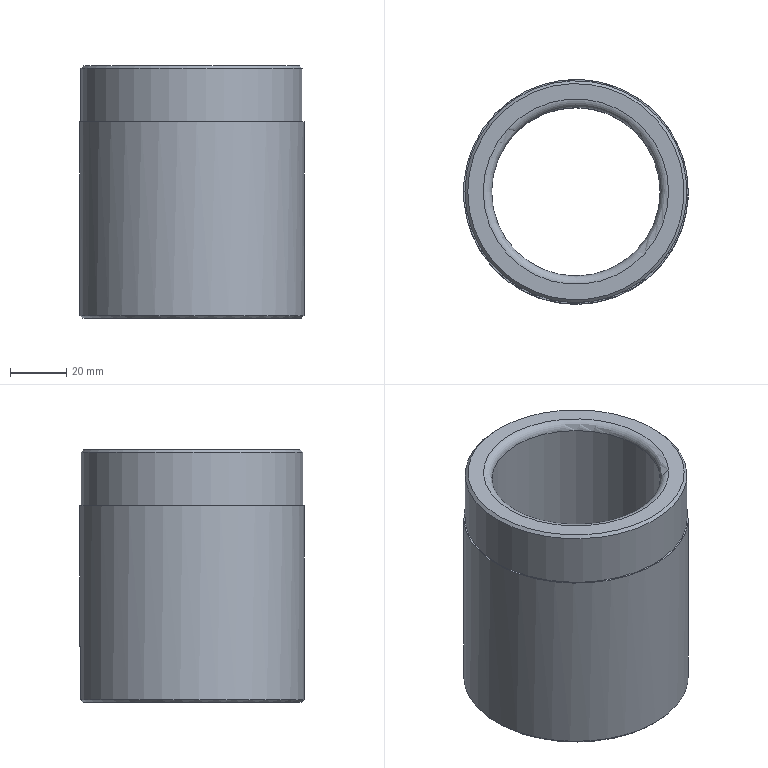Part | NX | features solid 2 | 1 solid | 13 faces | box 80 x 80 x 90 mm | volume 191386 mm3 | plane 4 | cylinder 4 | cone 3 | torus 2 | commonest cylinder face diameters 10 x1 60 x1 79 x1 80 x1
STEP:
#1=CARTESIAN_POINT('',(1292.,-185.,-190.));
#2=VERTEX_POINT('',#1);
#3=CARTESIAN_POINT('',(1325.,-185.,-190.));
#4=DIRECTION('',(0.,0.,-1.));
#5=DIRECTION('',(-1.,0.,0.));
#6=AXIS2_PLACEMENT_3D('',#3,#4,#5);
#7=CIRCLE('',#6,33.);
#8=EDGE_CURVE('',#2,#2,#7,.F.);
#9=ORIENTED_EDGE('',*,*,#8,.F.);
#10=EDGE_LOOP('',(#9));
#11=FACE_BOUND('',#10,.T.);
#12=CARTESIAN_POINT('',(1286.5,-185.,-190.));
#13=VERTEX_POINT('',#12);
#14=CARTESIAN_POINT('',(1325.,-185.,-190.));
#15=DIRECTION('',(0.,0.,-1.));
#16=DIRECTION('',(-1.,0.,0.));
#17=AXIS2_PLACEMENT_3D('',#14,#15,#16);
#18=CIRCLE('',#17,38.5);
#19=EDGE_CURVE('',#13,#13,#18,.T.);
#20=ORIENTED_EDGE('',*,*,#19,.F.);
#21=EDGE_LOOP('',(#20));
#22=FACE_BOUND('',#21,.T.);
#23=CARTESIAN_POINT('',(1325.,-185.,-190.));
#24=DIRECTION('',(0.,0.,1.));
#25=DIRECTION('',(-1.,0.,0.));
#26=AXIS2_PLACEMENT_3D('',#23,#24,#25);
#27=PLANE('',#26);
#28=ADVANCED_FACE('',(#11,#22),#27,.T.);
#29=CARTESIAN_POINT('',(1285.5,-185.,-191.));
#30=VERTEX_POINT('',#29);
#31=CARTESIAN_POINT('',(1325.,-185.,-191.));
#32=DIRECTION('',(0.,0.,-1.));
#33=DIRECTION('',(-1.,0.,0.));
#34=AXIS2_PLACEMENT_3D('',#31,#32,#33);
#35=CIRCLE('',#34,39.5);
#36=EDGE_CURVE('',#30,#30,#35,.F.);
#37=ORIENTED_EDGE('',*,*,#36,.F.);
#38=EDGE_LOOP('',(#37));
#39=FACE_BOUND('',#38,.T.);
#40=CARTESIAN_POINT('',(1285.5,-185.,-210.));
#41=VERTEX_POINT('',#40);
#42=CARTESIAN_POINT('',(1325.,-185.,-210.));
#43=DIRECTION('',(0.,0.,-1.));
#44=DIRECTION('',(-1.,0.,0.));
#45=AXIS2_PLACEMENT_3D('',#42,#43,#44);
#46=CIRCLE('',#45,39.5);
#47=EDGE_CURVE('',#41,#41,#46,.F.);
#48=ORIENTED_EDGE('',*,*,#47,.T.);
#49=EDGE_LOOP('',(#48));
#50=FACE_BOUND('',#49,.T.);
#51=CARTESIAN_POINT('',(1325.,-185.,-210.));
#52=DIRECTION('',(0.,0.,1.));
#53=DIRECTION('',(-1.,0.,0.));
#54=AXIS2_PLACEMENT_3D('',#51,#52,#53);
#55=CYLINDRICAL_SURFACE('',#54,39.5);
#56=ADVANCED_FACE('',(#39,#50),#55,.T.);
#57=ORIENTED_EDGE('',*,*,#47,.F.);
#58=EDGE_LOOP('',(#57));
#59=FACE_BOUND('',#58,.T.);
#60=CARTESIAN_POINT('',(1365.,-185.,-210.));
#61=VERTEX_POINT('',#60);
#62=CARTESIAN_POINT('',(1325.,-185.,-210.));
#63=DIRECTION('',(0.,0.,1.));
#64=DIRECTION('',(1.,0.,0.));
#65=AXIS2_PLACEMENT_3D('',#62,#63,#64);
#66=CIRCLE('',#65,40.);
#67=EDGE_CURVE('',#61,#61,#66,.T.);
#68=ORIENTED_EDGE('',*,*,#67,.T.);
#69=EDGE_LOOP('',(#68));
#70=FACE_BOUND('',#69,.T.);
#71=CARTESIAN_POINT('',(1325.,-185.,-210.));
#72=DIRECTION('',(0.,0.,1.));
#73=DIRECTION('',(-1.,0.,0.));
#74=AXIS2_PLACEMENT_3D('',#71,#72,#73);
#75=PLANE('',#74);
#76=ADVANCED_FACE('',(#59,#70),#75,.T.);
#77=CARTESIAN_POINT('',(1320.172,-146.3,-280.));
#78=VERTEX_POINT('',#77);
#79=CARTESIAN_POINT('',(1329.828,-146.3,-280.));
#80=VERTEX_POINT('',#79);
#81=CARTESIAN_POINT('',(1325.,-145.,-280.));
#82=DIRECTION('',(0.,0.,1.));
#83=DIRECTION('',(1.,0.,0.));
#84=AXIS2_PLACEMENT_3D('',#81,#82,#83);
#85=CIRCLE('',#84,5.);
#86=EDGE_CURVE('',#78,#80,#85,.T.);
#87=ORIENTED_EDGE('',*,*,#86,.T.);
#88=CARTESIAN_POINT('',(1325.,-185.,-280.));
#89=DIRECTION('',(0.,0.,1.));
#90=DIRECTION('',(1.,0.,0.));
#91=AXIS2_PLACEMENT_3D('',#88,#89,#90);
#92=CIRCLE('',#91,39.);
#93=EDGE_CURVE('',#78,#80,#92,.T.);
#94=ORIENTED_EDGE('',*,*,#93,.F.);
#95=EDGE_LOOP('',(#87,#94));
#96=FACE_BOUND('',#95,.T.);
#97=CARTESIAN_POINT('',(1292.321,-185.,-280.));
#98=VERTEX_POINT('',#97);
#99=CARTESIAN_POINT('',(1325.,-185.,-280.));
#100=DIRECTION('',(0.,0.,-1.));
#101=DIRECTION('',(-1.,0.,0.));
#102=AXIS2_PLACEMENT_3D('',#99,#100,#101);
#103=CIRCLE('',#102,32.679);
#104=EDGE_CURVE('',#98,#98,#103,.T.);
#105=ORIENTED_EDGE('',*,*,#104,.F.);
#106=EDGE_LOOP('',(#105));
#107=FACE_BOUND('',#106,.T.);
#108=CARTESIAN_POINT('',(1325.,-185.,-280.));
#109=DIRECTION('',(0.,0.,-1.));
#110=DIRECTION('',(1.,0.,0.));
#111=AXIS2_PLACEMENT_3D('',#108,#109,#110);
#112=PLANE('',#111);
#113=ADVANCED_FACE('',(#96,#107),#112,.T.);
#114=CARTESIAN_POINT('',(1329.99,-145.312,-279.));
#115=VERTEX_POINT('',#114);
#116=CARTESIAN_POINT('',(1329.99,-145.312,-260.));
#117=VERTEX_POINT('',#116);
#118=CARTESIAN_POINT('',(1329.99,-145.312,-270.));
#119=DIRECTION('',(0.,0.,1.));
#120=VECTOR('',#119,1000.);
#121=LINE('',#118,#120);
#122=EDGE_CURVE('',#115,#117,#121,.T.);
#123=ORIENTED_EDGE('',*,*,#122,.T.);
#124=CARTESIAN_POINT('',(1320.01,-145.312,-260.));
#125=VERTEX_POINT('',#124);
#126=CARTESIAN_POINT('',(1325.,-185.,-260.));
#127=DIRECTION('',(0.,0.,-1.));
#128=DIRECTION('',(-1.,0.,0.));
#129=AXIS2_PLACEMENT_3D('',#126,#127,#128);
#130=CIRCLE('',#129,40.);
#131=EDGE_CURVE('',#117,#125,#130,.F.);
#132=ORIENTED_EDGE('',*,*,#131,.T.);
#133=CARTESIAN_POINT('',(1320.01,-145.312,-279.));
#134=VERTEX_POINT('',#133);
#135=CARTESIAN_POINT('',(1320.01,-145.312,-270.));
#136=DIRECTION('',(0.,0.,1.));
#137=VECTOR('',#136,1000.);
#138=LINE('',#135,#137);
#139=EDGE_CURVE('',#125,#134,#138,.F.);
#140=ORIENTED_EDGE('',*,*,#139,.T.);
#141=CARTESIAN_POINT('',(1325.,-185.,-279.));
#142=DIRECTION('',(0.,0.,1.));
#143=DIRECTION('',(1.,0.,0.));
#144=AXIS2_PLACEMENT_3D('',#141,#142,#143);
#145=CIRCLE('',#144,40.);
#146=EDGE_CURVE('',#115,#134,#145,.F.);
#147=ORIENTED_EDGE('',*,*,#146,.F.);
#148=EDGE_LOOP('',(#123,#132,#140,#147));
#149=FACE_BOUND('',#148,.T.);
#150=ORIENTED_EDGE('',*,*,#67,.F.);
#151=EDGE_LOOP('',(#150));
#152=FACE_BOUND('',#151,.T.);
#153=CARTESIAN_POINT('',(1325.,-185.,-280.));
#154=DIRECTION('',(0.,0.,1.));
#155=DIRECTION('',(-1.,0.,0.));
#156=AXIS2_PLACEMENT_3D('',#153,#154,#155);
#157=CYLINDRICAL_SURFACE('',#156,40.);
#158=ADVANCED_FACE('',(#149,#152),#157,.T.);
#159=CARTESIAN_POINT('',(1295.,-185.,-193.));
#160=VERTEX_POINT('',#159);
#161=CARTESIAN_POINT('',(1325.,-185.,-193.));
#162=DIRECTION('',(0.,0.,-1.));
#163=DIRECTION('',(-1.,0.,0.));
#164=AXIS2_PLACEMENT_3D('',#161,#162,#163);
#165=CIRCLE('',#164,30.);
#166=EDGE_CURVE('',#160,#160,#165,.T.);
#167=ORIENTED_EDGE('',*,*,#166,.F.);
#168=EDGE_LOOP('',(#167));
#169=FACE_BOUND('',#168,.T.);
#170=CARTESIAN_POINT('',(1295.,-185.,-267.367));
#171=VERTEX_POINT('',#170);
#172=CARTESIAN_POINT('',(1325.,-185.,-267.367));
#173=DIRECTION('',(0.,0.,-1.));
#174=DIRECTION('',(-1.,0.,0.));
#175=AXIS2_PLACEMENT_3D('',#172,#173,#174);
#176=CIRCLE('',#175,30.);
#177=EDGE_CURVE('',#171,#171,#176,.F.);
#178=ORIENTED_EDGE('',*,*,#177,.F.);
#179=EDGE_LOOP('',(#178));
#180=FACE_BOUND('',#179,.T.);
#181=CARTESIAN_POINT('',(1325.,-185.,-285.));
#182=DIRECTION('',(0.,0.,1.));
#183=DIRECTION('',(-1.,0.,0.));
#184=AXIS2_PLACEMENT_3D('',#181,#182,#183);
#185=CYLINDRICAL_SURFACE('',#184,30.);
#186=ADVANCED_FACE('',(#169,#180),#185,.F.);
#187=CARTESIAN_POINT('',(1294.319,-185.,-272.543));
#188=VERTEX_POINT('',#187);
#189=CARTESIAN_POINT('',(1325.,-185.,-272.543));
#190=DIRECTION('',(0.,0.,-1.));
#191=DIRECTION('',(-1.,0.,0.));
#192=AXIS2_PLACEMENT_3D('',#189,#190,#191);
#193=CIRCLE('',#192,30.681);
#194=EDGE_CURVE('',#188,#188,#193,.T.);
#195=ORIENTED_EDGE('',*,*,#194,.F.);
#196=EDGE_LOOP('',(#195));
#197=FACE_BOUND('',#196,.T.);
#198=ORIENTED_EDGE('',*,*,#104,.T.);
#199=EDGE_LOOP('',(#198));
#200=FACE_BOUND('',#199,.T.);
#201=CARTESIAN_POINT('',(1325.,-185.,-270.));
#202=DIRECTION('',(0.,0.,-1.));
#203=DIRECTION('',(1.,0.,0.));
#204=AXIS2_PLACEMENT_3D('',#201,#202,#203);
#205=CONICAL_SURFACE('',#204,30.,0.2618);
#206=ADVANCED_FACE('',(#197,#200),#205,.F.);
#207=CARTESIAN_POINT('',(1320.01,-145.312,-279.));
#208=CARTESIAN_POINT('',(1320.031,-145.646,-279.334));
#209=CARTESIAN_POINT('',(1320.085,-145.976,-279.667));
#210=CARTESIAN_POINT('',(1320.172,-146.3,-280.));
#211=B_SPLINE_CURVE_WITH_KNOTS('',3,(#207,#208,#209,#210),.UNSPECIFIED.,.F.,.F.,(4,4),(0.000000282,0.001415),.UNSPECIFIED.);
#212=EDGE_CURVE('',#134,#78,#211,.T.);
#213=ORIENTED_EDGE('',*,*,#212,.T.);
#214=ORIENTED_EDGE('',*,*,#93,.T.);
#215=CARTESIAN_POINT('',(1329.828,-146.3,-280.));
#216=CARTESIAN_POINT('',(1329.915,-145.976,-279.667));
#217=CARTESIAN_POINT('',(1329.969,-145.646,-279.334));
#218=CARTESIAN_POINT('',(1329.99,-145.312,-279.));
#219=B_SPLINE_CURVE_WITH_KNOTS('',3,(#215,#216,#217,#218),.UNSPECIFIED.,.F.,.F.,(4,4),(0.000000284,0.001415),.UNSPECIFIED.);
#220=EDGE_CURVE('',#80,#115,#219,.T.);
#221=ORIENTED_EDGE('',*,*,#220,.T.);
#222=ORIENTED_EDGE('',*,*,#146,.T.);
#223=EDGE_LOOP('',(#213,#214,#221,#222));
#224=FACE_BOUND('',#223,.T.);
#225=CARTESIAN_POINT('',(1325.,-185.,-279.));
#226=DIRECTION('',(0.,0.,1.));
#227=DIRECTION('',(-1.,0.,0.));
#228=AXIS2_PLACEMENT_3D('',#225,#226,#227);
#229=CONICAL_SURFACE('',#228,40.,0.7854);
#230=ADVANCED_FACE('',(#224),#229,.T.);
#231=ORIENTED_EDGE('',*,*,#194,.T.);
#232=EDGE_LOOP('',(#231));
#233=FACE_BOUND('',#232,.T.);
#234=ORIENTED_EDGE('',*,*,#177,.T.);
#235=EDGE_LOOP('',(#234));
#236=FACE_BOUND('',#235,.T.);
#237=CARTESIAN_POINT('',(1325.,-185.,-267.367));
#238=DIRECTION('',(0.,0.,1.));
#239=DIRECTION('',(-1.,0.,0.));
#240=AXIS2_PLACEMENT_3D('',#237,#238,#239);
#241=TOROIDAL_SURFACE('',#240,50.,20.);
#242=ADVANCED_FACE('',(#233,#236),#241,.T.);
#243=ORIENTED_EDGE('',*,*,#19,.T.);
#244=EDGE_LOOP('',(#243));
#245=FACE_BOUND('',#244,.T.);
#246=ORIENTED_EDGE('',*,*,#36,.T.);
#247=EDGE_LOOP('',(#246));
#248=FACE_BOUND('',#247,.T.);
#249=CARTESIAN_POINT('',(1325.,-185.,-191.));
#250=DIRECTION('',(0.,0.,-1.));
#251=DIRECTION('',(1.,0.,0.));
#252=AXIS2_PLACEMENT_3D('',#249,#250,#251);
#253=CONICAL_SURFACE('',#252,39.5,0.7854);
#254=ADVANCED_FACE('',(#245,#248),#253,.T.);
#255=ORIENTED_EDGE('',*,*,#166,.T.);
#256=EDGE_LOOP('',(#255));
#257=FACE_BOUND('',#256,.T.);
#258=ORIENTED_EDGE('',*,*,#8,.T.);
#259=EDGE_LOOP('',(#258));
#260=FACE_BOUND('',#259,.T.);
#261=CARTESIAN_POINT('',(1325.,-185.,-193.));
#262=DIRECTION('',(0.,0.,1.));
#263=DIRECTION('',(-1.,0.,0.));
#264=AXIS2_PLACEMENT_3D('',#261,#262,#263);
#265=TOROIDAL_SURFACE('',#264,33.,3.);
#266=ADVANCED_FACE('',(#257,#260),#265,.T.);
#267=ORIENTED_EDGE('',*,*,#139,.F.);
#268=CARTESIAN_POINT('',(1325.,-145.,-260.));
#269=DIRECTION('',(0.,0.,1.));
#270=DIRECTION('',(1.,0.,0.));
#271=AXIS2_PLACEMENT_3D('',#268,#269,#270);
#272=CIRCLE('',#271,5.);
#273=EDGE_CURVE('',#125,#117,#272,.T.);
#274=ORIENTED_EDGE('',*,*,#273,.T.);
#275=ORIENTED_EDGE('',*,*,#122,.F.);
#276=ORIENTED_EDGE('',*,*,#220,.F.);
#277=ORIENTED_EDGE('',*,*,#86,.F.);
#278=ORIENTED_EDGE('',*,*,#212,.F.);
#279=EDGE_LOOP('',(#267,#274,#275,#276,#277,#278));
#280=FACE_BOUND('',#279,.T.);
#281=CARTESIAN_POINT('',(1325.,-145.,-280.));
#282=DIRECTION('',(0.,0.,1.));
#283=DIRECTION('',(1.,0.,0.));
#284=AXIS2_PLACEMENT_3D('',#281,#282,#283);
#285=CYLINDRICAL_SURFACE('',#284,5.);
#286=ADVANCED_FACE('',(#280),#285,.F.);
#287=ORIENTED_EDGE('',*,*,#131,.F.);
#288=ORIENTED_EDGE('',*,*,#273,.F.);
#289=EDGE_LOOP('',(#287,#288));
#290=FACE_BOUND('',#289,.T.);
#291=CARTESIAN_POINT('',(1325.,-145.,-260.));
#292=DIRECTION('',(0.,0.,1.));
#293=DIRECTION('',(1.,0.,0.));
#294=AXIS2_PLACEMENT_3D('',#291,#292,#293);
#295=PLANE('',#294);
#296=ADVANCED_FACE('',(#290),#295,.F.);
#297=CLOSED_SHELL('',(#28,#56,#76,#113,#158,#186,#206,#230,#242,#254,#266,#286,#296));
#298=MANIFOLD_SOLID_BREP('',#297);
#299=(LENGTH_UNIT()NAMED_UNIT(*)SI_UNIT(.MILLI.,.METRE.));
#300=UNCERTAINTY_MEASURE_WITH_UNIT(LENGTH_MEASURE(0.0508),#299,'','');
#301=(NAMED_UNIT(*)PLANE_ANGLE_UNIT()SI_UNIT($,.RADIAN.));
#302=(NAMED_UNIT(*)SI_UNIT($,.STERADIAN.)SOLID_ANGLE_UNIT());
#303=(GEOMETRIC_REPRESENTATION_CONTEXT(3)GLOBAL_UNCERTAINTY_ASSIGNED_CONTEXT((#300))GLOBAL_UNIT_ASSIGNED_CONTEXT((#299,#301,#302))REPRESENTATION_CONTEXT('',''));
#304=ADVANCED_BREP_SHAPE_REPRESENTATION('',(#298),#303);